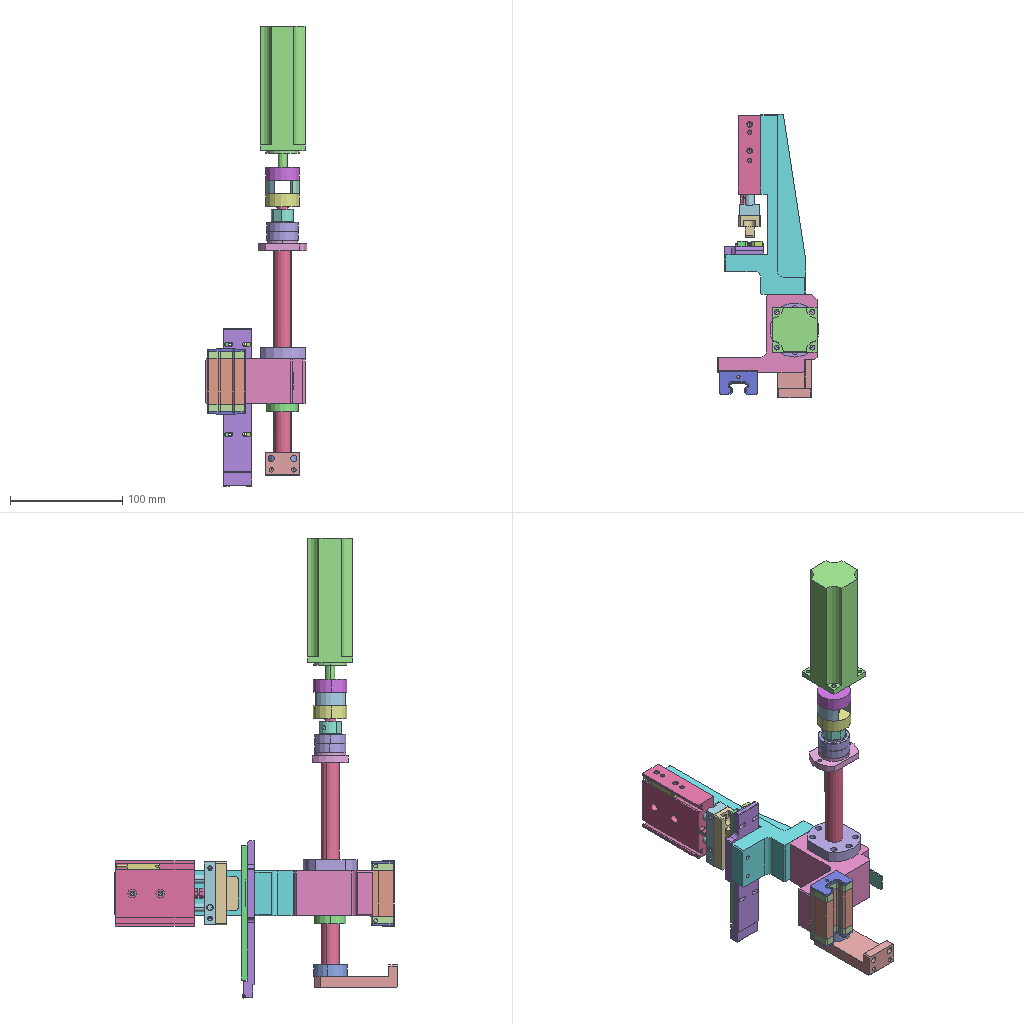Assembly | SolidWorks | 33 different items | 42 placed | box 91 x 252 x 409 mm
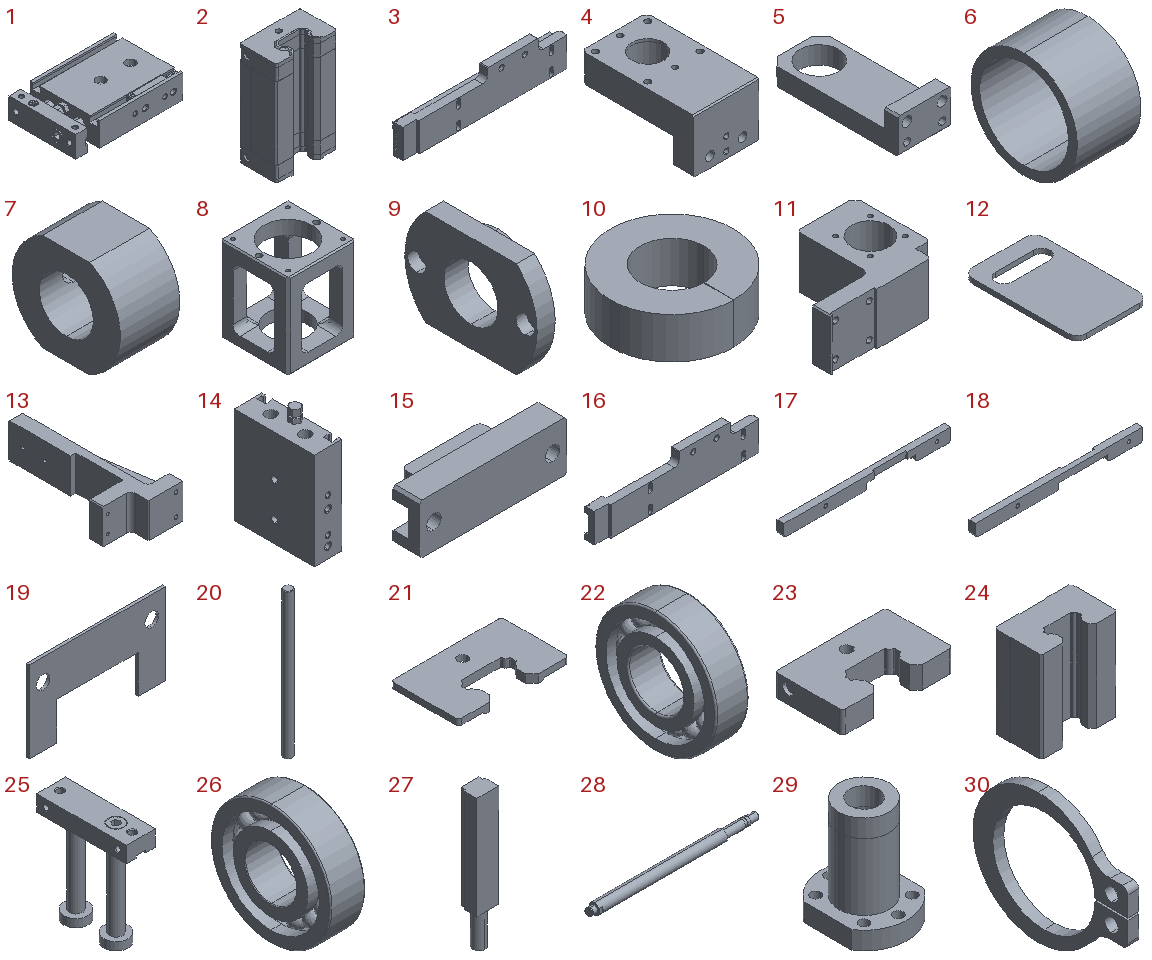Parts list (item | name | quantity | parent item | size | volume | features):
1 | (subassembly) | x1 | - | 89 x 58 x 20 mm | 84198 mm3 | features AEMSimFeature 1
2 | (subassembly) | x1 | - | 34 x 21 x 58.6 mm | 32343 mm3 | -
3 | (subassembly) | x1 | - | 140 x 12 x 35 mm | 35220 mm3 | features AEMSimFeature 1, CompositeCurve 1
4 | - | x1 | - | 50 x 86 x 41 mm | 88498 mm3 | features HoleWzd 4, ICE 3, Chamfer 2, Extrusion 1
5 | - | x1 | - | 30 x 74 x 20 mm | 19884 mm3 | features Chamfer 2, ICE 2, Extrusion 1, HoleWzd 1
6 | - | x1 | - | 9 x 15 x 15 mm | 485.965 mm3 | features Revolution 1
7 | - | x1 | - | 12 x 20 x 18 mm | 2542 mm3 | features HoleWzd 1, ICE 1, Revolution 1
8 | - | x1 | - | 50 x 50 x 62 mm | 46792 mm3 | features HoleWzd 3, ICE 3, Chamfer 2, CirPattern 1, Extrusion 1, Fillet 1, RefAxis 1
9 | - | x1 | - | 9 x 44 x 32 mm | 6703 mm3 | features HoleWzd 1, ICE 1, Revolution 1
10 | - | x1 | - | 30 x 30 x 10 mm | 5174 mm3 | features Extrusion 1, ICE 1
11 | - | x1 | - | 89 x 70 x 40 mm | 113101 mm3 | features HoleWzd 5, Chamfer 3, ICE 3, Extrusion 1, Fillet 1
12 | - | x1 | - | 15 x 24 x 1 mm | 318.945 mm3 | features Extrusion 1, Fillet 1
13 | - | x1 | - | 72.5 x 160 x 40 mm | 135380 mm3 | features HoleWzd 3, ICE 3, Fillet 2, Chamfer 1, Extrusion 1
14 | - | x1 | in 1 | 20 x 58 x 79 mm | 67416 mm3 | features HoleWzd 10, RefAxis 9, RevCut 4, 3DProfileFeature 3, Revolution 2, Extrusion 1, ICE 1
15 | - | x1 | - | 56 x 20 x 19 mm | 11727 mm3 | features ICE 2, Chamfer 1, Extrusion 1, Fillet 1, HoleWzd 1
16 | - | x1 | in 3 | 140 x 10 x 35 mm | 26170 mm3 | features ICE 6, CutThin 5, HoleWzd 3, Emboss 2, Fillet 2, LPattern 2, MirrorPattern 2, Chamfer 1, Extrusion 1
17 | - | x1 | in 3 | 120 x 5 x 9 mm | 4384 mm3 | features Fillet 2, ICE 2, Extrusion 1, HoleWzd 1
18 | - | x1 | in 3 | 120 x 5 x 9 mm | 4384 mm3 | features Fillet 2, ICE 2, Extrusion 1, HoleWzd 1
19 | - | x1 | in 3 | 25 x 0.5 x 15 mm | 130.091 mm3 | features Extrusion 1
20 | - | x1 | in 3 | 1.5 x 1.5 x 25 mm | 44.134 mm3 | features Chamfer 1, Extrusion 1
21 | - | x2 | in 2 | 33.5 x 20.5 x 2.5 mm | 1023 mm3 | features BaseBody 1
22 | - | x1 | - | 6 x 22 x 22 mm | 1339 mm3 | features MoveCopyBody 1, Stock 1
23 | - | x2 | in 2 | 33.5 x 20.5 x 6.7 mm | 3669 mm3 | features BaseBody 1
24 | - | x1 | in 2 | 34 x 21 x 40.2 mm | 22959 mm3 | features BaseBody 1
25 | - | x1 | in 1 | 18 x 56 x 64 mm | 15836 mm3 | features ICE 5, HoleWzd 4, RefAxis 3, RevCut 2, Revolution 2, 3DProfileFeature 1, Extrusion 1
26 | - | x2 | - | 8 x 28 x 28 mm | 2884 mm3 | features Stock 1
27 | - | x1 | in 1 | 6.2 x 5 x 39 mm | 946.118 mm3 | features RefAxis 6, 3DProfileFeature 2, Extrusion 1, RevCut 1, Revolution 1
28 | - | x1 | - | 250 x 16 x 16 mm | 43988 mm3 | features Chamfer 1, ICE 1, Revolution 1
29 | - | x1 | - | 40 x 48 x 57 mm | 32709 mm3 | features Extrusion 1, HoleWzd 1, ICE 1, MirrorPattern 1, Split 1
30 | - | x1 | - | 1 x 14.1 x 11.82 mm | 51.029 mm3 | features RefAxis 3, 3DProfileFeature 1, Extrusion 1
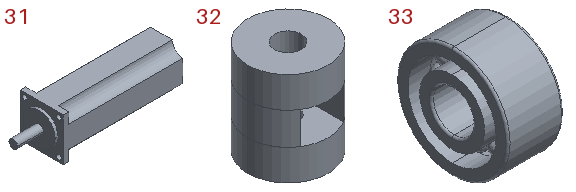31 | - | x1 | - | 137.2 x 40 x 40 mm | 146758 mm3 | features ICE 3, CirPattern 1, Extrusion 1, HoleWzd 1
32 | - | x1 | - | 30 x 30 x 35 mm | 17785 mm3 | features ICE 2, Extrusion 1, Split 1
33 | - | x7 | in 3 | 2 x 4 x 4 mm | 15.38 mm3 | features MoveCopyBody 1, Stock 1
Mates (type | each side: item.copy, entity, surface, feature):
In the top assembly
Coincident | 4.1 face plane Boss-Extrude1 | 9.1 face plane Revolve1
Concentric | 4.1 face cylinder M3 Tapped Hole1 | 9.1 face cylinder CBORE for M3 Hex Head Bolt1
Coincident | 5.1 face plane Boss-Extrude1 | 10.1 face plane Boss-Extrude1
Concentric | 28.1 face cylinder Revolve1 | 10.1 face cylinder Boss-Extrude1
Concentric | 28.1 face cylinder Revolve1 | 6.1 face cylinder Revolve1
Coincident | 28.1 face plane Revolve1 | 6.1 face plane Revolve1
Concentric | 28.1 face cylinder Revolve1 | 9.1 face cylinder Revolve1
LimitDistanceDim | 29.1 face plane Boss-Extrude1 | 9.1 face plane Revolve1
Concentric | 28.1 face cylinder Revolve1 | 7.1 face cylinder Revolve1
Concentric | 29.1 face cylinder Boss-Extrude1 | 28.1 face cylinder Revolve1
Concentric | 28.1 face cylinder Revolve1 | 32.1 face cylinder Boss-Extrude1
Coincident | 28.1 face plane Revolve1 | 32.1 face plane Cut-Extrude1
Coincident | 24.1 face plane Input 1 | 11.1 face plane Cut-Extrude1
Concentric | 24.1 face cylinder Input 1 | 11.1 face cylinder Ø4.5 (4.5) Diameter Hole1 | 2 times
Concentric | 29.1 face cylinder Boss-Extrude1 | 11.1 face cylinder Boss-Extrude1
Coincident | 29.1 face plane Boss-Extrude2 | 11.1 face plane Boss-Extrude1
Concentric | 29.1 face cylinder Ø5.5 (5.5) Diameter Hole1 | 11.1 face cylinder M4 Tapped Hole1
Coincident | 13.1 face plane Boss-Extrude1 | 16.1 face plane Boss-Extrude1
Concentric | 13.1 face cylinder M4 Tapped Hole1 | 16.1 face cylinder Hole size per socket head cap screw type 2 | 2 times
Parallel | 4.1 face plane Boss-Extrude1 | 11.1 face plane Boss-Extrude1
Concentric | 11.1 face cylinder M5 Tapped Hole1 | 13.1 face cylinder Cut-Extrude2 | 2 times
Coincident | 11.1 face plane Boss-Extrude1 | 13.1 face plane Boss-Extrude1
Coincident | 11.1 face plane Cut-Extrude2 | 12.1 face plane Boss-Extrude1
DistanceDim | 12.1 face plane Boss-Extrude1 | 11.1 face plane Boss-Extrude1 | 2 times
Concentric | 28.1 face cylinder Revolve1 | 22.1 face cylinder deep groove ball bearings gb
Coincident | 28.1 face plane Revolve1 | 22.1 face plane deep groove ball bearings gb
Concentric | 28.1 face cylinder Revolve1 | 26.1 face cylinder angular contact ball bearings gb
Coincident | 6.1 face plane Revolve1 | 26.1 face plane angular contact ball bearings gb
Concentric | 28.1 face cylinder Revolve1 | 26.2 face cylinder angular contact ball bearings gb
Coincident | 26.1 face plane angular contact ball bearings gb | 26.2 face plane angular contact ball bearings gb
Coincident | 7.1 face plane Revolve1 | 26.2 face plane angular contact ball bearings gb
Coincident | 9.1 face plane Revolve1 | 26.1 face plane angular contact ball bearings gb
Coincident | 5.1 face plane Boss-Extrude1 | 22.1 face plane deep groove ball bearings gb
Concentric | 5.1 face cylinder Boss-Extrude1 | 22.1 face cylinder deep groove ball bearings gb
Concentric | 4.1 face cylinder Boss-Extrude1 | 26.1 face cylinder angular contact ball bearings gb
Concentric | 31.1 face cylinder Boss-Extrude2 | 8.1 face cylinder Boss-Extrude1
Coincident | 31.1 face plane Boss-Extrude1 | 8.1 face plane Boss-Extrude1
Concentric | 28.1 face cylinder Revolve1 | 8.1 face cylinder Cut-Extrude1
Concentric | 4.1 face cylinder Ø4.0 (4) Diameter Hole2 | 8.1 face cylinder Ø4.0 (4) Diameter Hole1
Coincident | 4.1 face plane Boss-Extrude1 | 8.1 face plane Boss-Extrude1
Concentric | 31.1 face cylinder CirPattern1 | 8.1 face cylinder M4 Tapped Hole1
Coincident | 13.1 face plane Boss-Extrude1 | 14.1 face plane Boss-Extrude1
Concentric | 13.1 face cylinder M4 Tapped Hole2 | 14.1 face cylinder Hole2
Concentric | 13.1 face cylinder M4 Tapped Hole2 | 14.1 face cylinder Hole1
Coincident | 15.1 face plane Boss-Extrude1 | 25.1 face plane Boss-Extrude1
Concentric | 15.1 face cylinder Hole size per socket head cap screw type 1 | 25.1 face cylinder Cut-Revolve1
Concentric | 15.1 face cylinder Hole size per socket head cap screw type 1 | 25.1 face cylinder Cut-Revolve2
Concentric | 28.1 face cylinder Revolve1 | 30.1 face cylinder Boss-Extrude1
Coincident | 28.1 face plane Revolve1 | 30.1 face plane Boss-Extrude1
In subassembly 1
Coincident | 14.2 axis | 25.2 axis
PlanarAngleDim | 25.2 plane | 14.2 plane
Coincident | 14.2 axis | 27.1 axis
In subassembly 3
Coincident | 16.2 face plane Cut-Extrude1 | 17.1 face plane Boss-Extrude1
DistanceDim | 16.2 face plane Cut-Extrude1 | 17.1 face plane Boss-Extrude1
Concentric | 16.2 face cylinder Cut-Extrude3 | 20.1 face cylinder Boss-Extrude1
Coincident | 16.2 face plane Boss-Extrude1 | 20.1 face plane Boss-Extrude1
Coincident | 16.2 face plane Boss-Extrude1 | 19.1 face plane Boss-Extrude1
Concentric | 16.2 face cylinder M2 Tapped Hole1 | 19.1 face cylinder Boss-Extrude1 | 2 times
Concentric | 20.1 face cylinder Boss-Extrude1 | 33.1 face cylinder 68-1.5ZZ Deep Groove Ball Bearing GB
Concentric | 20.1 face cylinder Boss-Extrude1 | 33.2 face cylinder 68-1.5ZZ Deep Groove Ball Bearing GB
Concentric | 20.1 face cylinder Boss-Extrude1 | 33.3 face cylinder 68-1.5ZZ Deep Groove Ball Bearing GB
Concentric | 20.1 face cylinder Boss-Extrude1 | 33.4 face cylinder 68-1.5ZZ Deep Groove Ball Bearing GB
Concentric | 20.1 face cylinder Boss-Extrude1 | 33.5 face cylinder 68-1.5ZZ Deep Groove Ball Bearing GB
Concentric | 20.1 face cylinder Boss-Extrude1 | 33.6 face cylinder 68-1.5ZZ Deep Groove Ball Bearing GB
Coincident | 16.2 face plane Cut-Extrude1 | 18.1 face plane Boss-Extrude1
Coincident | 17.1 face plane Boss-Extrude1 | 18.1 face plane Boss-Extrude1
Concentric | 20.1 face cylinder Boss-Extrude1 | 33.7 face cylinder 68-1.5ZZ Deep Groove Ball Bearing GB
Coincident | 33.4 face plane 68-1.5ZZ Deep Groove Ball Bearing GB | 33.6 face plane 68-1.5ZZ Deep Groove Ball Bearing GB
Coincident | 33.5 face plane 68-1.5ZZ Deep Groove Ball Bearing GB | 33.6 face plane 68-1.5ZZ Deep Groove Ball Bearing GB
Coincident | 33.5 face plane 68-1.5ZZ Deep Groove Ball Bearing GB | 33.2 face plane 68-1.5ZZ Deep Groove Ball Bearing GB
Coincident | 33.2 face plane 68-1.5ZZ Deep Groove Ball Bearing GB | 33.7 face plane 68-1.5ZZ Deep Groove Ball Bearing GB
Coincident | 33.1 face plane 68-1.5ZZ Deep Groove Ball Bearing GB | 33.7 edge
Coincident | 33.3 face plane 68-1.5ZZ Deep Groove Ball Bearing GB | 33.1 face plane 68-1.5ZZ Deep Groove Ball Bearing GB
DistanceDim | 33.3 face plane 68-1.5ZZ Deep Groove Ball Bearing GB | 16.2 face plane Cut-Extrude2